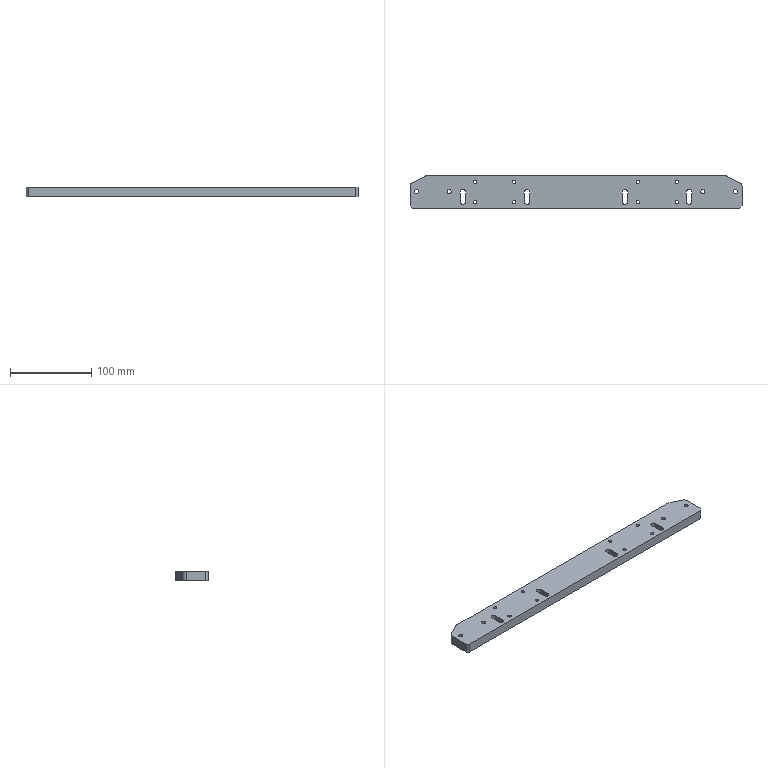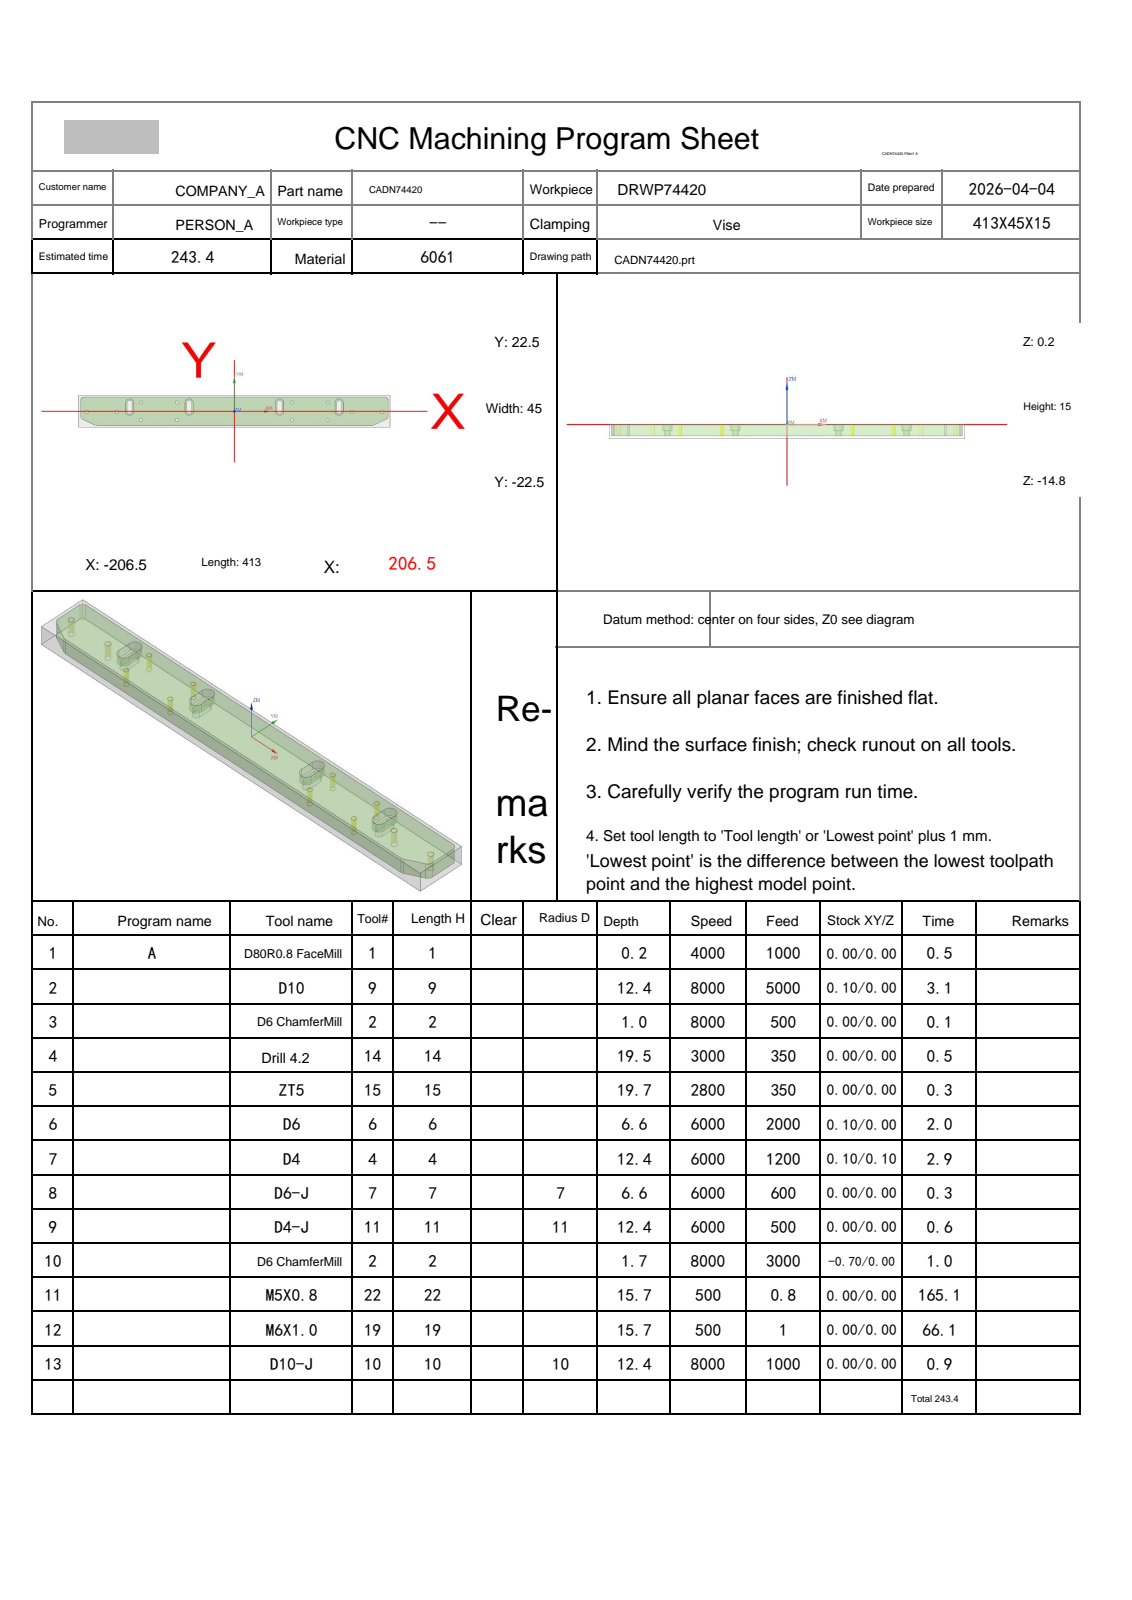NC program | NX | posted by the shop | part box 408 x 40 x 12 mm
Lines 1 to 1071 of 2398:
%
O0001
(Machine time: 462.93 MIN)
(===Total Tool:12===)
(T1=D80R0.8 FaceMill D=80.  R=0.8  D-  H01 Z=0.    )
(T9=D10     D=10.  R=0.   D-  H09 Z=-12.2 )
(T2=D6 ChamferMill   D=6.   R=0.   D-  H02 Z=-1.5  )
(T14=Drill 4.2  D=4.2  DR_a=118 D-  H14 Z=-19.26)
(T15=ZT5    D=5.   DR_a=118 D-  H15 Z=-19.5 )
(T6=D6      D=6.   R=0.   D-  H06 Z=-6.4  )
(T4=D4      D=4.   R=0.   D-  H04 Z=-12.2 )
(T7=D6-J    D=6.   R=0.   D7  H07 Z=-6.4  )
(T11=D4-J   D=4.   R=0.   D11 H11 Z=-12.2 )
(T22=M5X0.8 D=4.2  DR_a=180 D-  H22 Z=-15.5 )
(T19=M6X1.0 D=5.   DR_a=180 D-  H19 Z=-15.5 )
(T10=D10-J  D=10.  R=0.   D10 H10 Z=-12.2 )
G80 G90 G17 G49 G40
G91 G28 Z0
M01
N1 T01 M06
(D80R0.8 FaceMill  D=80. R=0.8 H=01 ce=0.00 di=0.00)
G00 G90 G54 X249. Y0.0 M03 S4000
G43 H01 Z20.
M08
Z2.
G01 Z0.0 F1000.
X244.
X-244.
X-249.
Z2.
G00 Z20.
G91 G28 Z0.0
M05
M09
G91 G28 Z0.0
M01
N2 T09 M06
(D10  D=10. R=0. H=09 ce=0.10 di=0.00)
G00 G90 G54 X0.0 Y25.1 M03 S8000
G43 H09 Z20.
M08
Z.5
G01 X201. Z.324 F5000.
G02 X204.606 Y23.606 Z.321 I0.0 J-5.1
G01 X207.606 Y20.606 Z.317
G02 X209.1 Y17. Z.314 I-3.606 J-3.606
G01 Y-6.91 Z.293
G02 X203.517 Y-15.944 Z.283 I-10.1 J0.0
G01 X187.337 Y-24.034 Z.267
G02 X182.82 Y-25.1 Z.263 I-4.517 J9.034
G01 X-182.82 Z-.057
G02 X-187.337 Y-24.034 Z-.061 I0.0 J10.1
G01 X-203.517 Y-15.944 Z-.077
G02 X-209.1 Y-6.91 Z-.086 I4.517 J9.034
G01 Y17. Z-.107
G02 X-207.606 Y20.606 Z-.111 I5.1 J0.0
G01 X-204.606 Y23.606 Z-.115
G02 X-201. Y25.1 Z-.118 I3.606 J-3.606
G01 X201. Z-.469
G02 X204.606 Y23.606 Z-.473 I0.0 J-5.1
G01 X207.606 Y20.606 Z-.477
G02 X209.1 Y17. Z-.48 I-3.606 J-3.606
G01 Y-6.91 Z-.501
G02 X203.517 Y-15.944 Z-.511 I-10.1 J0.0
G01 X187.337 Y-24.034 Z-.527
G02 X182.82 Y-25.1 Z-.531 I-4.517 J9.034
G01 X-182.82 Z-.85
G02 X-187.337 Y-24.034 Z-.855 I0.0 J10.1
G01 X-203.517 Y-15.944 Z-.87
G02 X-209.1 Y-6.91 Z-.88 I4.517 J9.034
G01 Y17. Z-.901
G02 X-207.606 Y20.606 Z-.905 I5.1 J0.0
G01 X-204.606 Y23.606 Z-.908
G02 X-201. Y25.1 Z-.912 I3.606 J-3.606
G01 X201. Z-1.263
G02 X204.606 Y23.606 Z-1.267 I0.0 J-5.1
G01 X207.606 Y20.606 Z-1.27
G02 X209.1 Y17. Z-1.274 I-3.606 J-3.606
G01 Y-6.91 Z-1.295
G02 X203.517 Y-15.944 Z-1.305 I-10.1 J0.0
G01 X187.337 Y-24.034 Z-1.32
G02 X182.82 Y-25.1 Z-1.325 I-4.517 J9.034
G01 X-182.82 Z-1.644
G02 X-187.337 Y-24.034 Z-1.648 I0.0 J10.1
G01 X-203.517 Y-15.944 Z-1.664
G02 X-209.1 Y-6.91 Z-1.674 I4.517 J9.034
G01 Y17. Z-1.695
G02 X-207.606 Y20.606 Z-1.698 I5.1 J0.0
G01 X-204.606 Y23.606 Z-1.702
G02 X-201. Y25.1 Z-1.706 I3.606 J-3.606
G01 X201. Z-2.057
G02 X204.606 Y23.606 Z-2.06 I0.0 J-5.1
G01 X207.606 Y20.606 Z-2.064
G02 X209.1 Y17. Z-2.068 I-3.606 J-3.606
G01 Y-6.91 Z-2.089
G02 X203.517 Y-15.944 Z-2.098 I-10.1 J0.0
G01 X187.337 Y-24.034 Z-2.114
G02 X182.82 Y-25.1 Z-2.118 I-4.517 J9.034
G01 X-182.82 Z-2.438
G02 X-187.337 Y-24.034 Z-2.442 I0.0 J10.1
G01 X-203.517 Y-15.944 Z-2.458
G02 X-209.1 Y-6.91 Z-2.468 I4.517 J9.034
G01 Y17. Z-2.489
G02 X-207.606 Y20.606 Z-2.492 I5.1 J0.0
G01 X-204.606 Y23.606 Z-2.496
G02 X-201. Y25.1 Z-2.499 I3.606 J-3.606
G01 X201. Z-2.851
G02 X204.606 Y23.606 Z-2.854 I0.0 J-5.1
G01 X207.606 Y20.606 Z-2.858
G02 X209.1 Y17. Z-2.861 I-3.606 J-3.606
G01 Y-6.91 Z-2.882
G02 X203.517 Y-15.944 Z-2.892 I-10.1 J0.0
G01 X187.337 Y-24.034 Z-2.908
G02 X182.82 Y-25.1 Z-2.912 I-4.517 J9.034
G01 X-182.82 Z-3.232
G02 X-187.337 Y-24.034 Z-3.236 I0.0 J10.1
G01 X-203.517 Y-15.944 Z-3.252
G02 X-209.1 Y-6.91 Z-3.261 I4.517 J9.034
G01 Y17. Z-3.282
G02 X-207.606 Y20.606 Z-3.286 I5.1 J0.0
G01 X-204.606 Y23.606 Z-3.29
G02 X-201. Y25.1 Z-3.293 I3.606 J-3.606
G01 X201. Z-3.644
G02 X204.606 Y23.606 Z-3.648 I0.0 J-5.1
G01 X207.606 Y20.606 Z-3.652
G02 X209.1 Y17. Z-3.655 I-3.606 J-3.606
G01 Y-6.91 Z-3.676
G02 X203.517 Y-15.944 Z-3.686 I-10.1 J0.0
G01 X187.337 Y-24.034 Z-3.702
G02 X182.82 Y-25.1 Z-3.706 I-4.517 J9.034
G01 X-182.82 Z-4.025
G02 X-187.337 Y-24.034 Z-4.03 I0.0 J10.1
G01 X-203.517 Y-15.944 Z-4.045
G02 X-209.1 Y-6.91 Z-4.055 I4.517 J9.034
G01 Y17. Z-4.076
G02 X-207.606 Y20.606 Z-4.08 I5.1 J0.0
G01 X-204.606 Y23.606 Z-4.083
G02 X-201. Y25.1 Z-4.087 I3.606 J-3.606
G01 X201. Z-4.438
G02 X204.606 Y23.606 Z-4.442 I0.0 J-5.1
G01 X207.606 Y20.606 Z-4.445
G02 X209.1 Y17. Z-4.449 I-3.606 J-3.606
G01 Y-6.91 Z-4.47
G02 X203.517 Y-15.944 Z-4.48 I-10.1 J0.0
G01 X187.337 Y-24.034 Z-4.495
G02 X182.82 Y-25.1 Z-4.5 I-4.517 J9.034
G01 X-182.82 Z-4.819
G02 X-187.337 Y-24.034 Z-4.823 I0.0 J10.1
G01 X-203.517 Y-15.944 Z-4.839
G02 X-209.1 Y-6.91 Z-4.849 I4.517 J9.034
G01 Y17. Z-4.87
G02 X-207.606 Y20.606 Z-4.873 I5.1 J0.0
G01 X-204.606 Y23.606 Z-4.877
G02 X-201. Y25.1 Z-4.881 I3.606 J-3.606
G01 X201. Z-5.232
G02 X204.606 Y23.606 Z-5.235 I0.0 J-5.1
G01 X207.606 Y20.606 Z-5.239
G02 X209.1 Y17. Z-5.243 I-3.606 J-3.606
G01 Y-6.91 Z-5.264
G02 X203.517 Y-15.944 Z-5.273 I-10.1 J0.0
G01 X187.337 Y-24.034 Z-5.289
G02 X182.82 Y-25.1 Z-5.293 I-4.517 J9.034
G01 X-182.82 Z-5.613
G02 X-187.337 Y-24.034 Z-5.617 I0.0 J10.1
G01 X-203.517 Y-15.944 Z-5.633
G02 X-209.1 Y-6.91 Z-5.643 I4.517 J9.034
G01 Y17. Z-5.664
G02 X-207.606 Y20.606 Z-5.667 I5.1 J0.0
G01 X-204.606 Y23.606 Z-5.671
G02 X-201. Y25.1 Z-5.674 I3.606 J-3.606
G01 X201. Z-6.026
G02 X204.606 Y23.606 Z-6.029 I0.0 J-5.1
G01 X207.606 Y20.606 Z-6.033
G02 X209.1 Y17. Z-6.036 I-3.606 J-3.606
G01 Y-6.91 Z-6.057
G02 X203.517 Y-15.944 Z-6.067 I-10.1 J0.0
G01 X187.337 Y-24.034 Z-6.083
G02 X182.82 Y-25.1 Z-6.087 I-4.517 J9.034
G01 X-182.82 Z-6.407
G02 X-187.337 Y-24.034 Z-6.411 I0.0 J10.1
G01 X-203.517 Y-15.944 Z-6.427
G02 X-209.1 Y-6.91 Z-6.436 I4.517 J9.034
G01 Y17. Z-6.457
G02 X-207.606 Y20.606 Z-6.461 I5.1 J0.0
G01 X-204.606 Y23.606 Z-6.465
G02 X-201. Y25.1 Z-6.468 I3.606 J-3.606
G01 X201. Z-6.819
G02 X204.606 Y23.606 Z-6.823 I0.0 J-5.1
G01 X207.606 Y20.606 Z-6.827
G02 X209.1 Y17. Z-6.83 I-3.606 J-3.606
G01 Y-6.91 Z-6.851
G02 X203.517 Y-15.944 Z-6.861 I-10.1 J0.0
G01 X187.337 Y-24.034 Z-6.877
G02 X182.82 Y-25.1 Z-6.881 I-4.517 J9.034
G01 X-182.82 Z-7.2
G02 X-187.337 Y-24.034 Z-7.205 I0.0 J10.1
G01 X-203.517 Y-15.944 Z-7.22
G02 X-209.1 Y-6.91 Z-7.23 I4.517 J9.034
G01 Y17. Z-7.251
G02 X-207.606 Y20.606 Z-7.255 I5.1 J0.0
G01 X-204.606 Y23.606 Z-7.258
G02 X-201. Y25.1 Z-7.262 I3.606 J-3.606
G01 X201. Z-7.613
G02 X204.606 Y23.606 Z-7.617 I0.0 J-5.1
G01 X207.606 Y20.606 Z-7.62
G02 X209.1 Y17. Z-7.624 I-3.606 J-3.606
G01 Y-6.91 Z-7.645
G02 X203.517 Y-15.944 Z-7.655 I-10.1 J0.0
G01 X187.337 Y-24.034 Z-7.67
G02 X182.82 Y-25.1 Z-7.675 I-4.517 J9.034
G01 X-182.82 Z-7.994
G02 X-187.337 Y-24.034 Z-7.998 I0.0 J10.1
G01 X-203.517 Y-15.944 Z-8.014
G02 X-209.1 Y-6.91 Z-8.024 I4.517 J9.034
G01 Y17. Z-8.045
G02 X-207.606 Y20.606 Z-8.048 I5.1 J0.0
G01 X-204.606 Y23.606 Z-8.052
G02 X-201. Y25.1 Z-8.056 I3.606 J-3.606
G01 X201. Z-8.407
G02 X204.606 Y23.606 Z-8.41 I0.0 J-5.1
G01 X207.606 Y20.606 Z-8.414
G02 X209.1 Y17. Z-8.418 I-3.606 J-3.606
G01 Y-6.91 Z-8.439
G02 X203.517 Y-15.944 Z-8.448 I-10.1 J0.0
G01 X187.337 Y-24.034 Z-8.464
G02 X182.82 Y-25.1 Z-8.468 I-4.517 J9.034
G01 X-182.82 Z-8.788
G02 X-187.337 Y-24.034 Z-8.792 I0.0 J10.1
G01 X-203.517 Y-15.944 Z-8.808
G02 X-209.1 Y-6.91 Z-8.818 I4.517 J9.034
G01 Y17. Z-8.839
G02 X-207.606 Y20.606 Z-8.842 I5.1 J0.0
G01 X-204.606 Y23.606 Z-8.846
G02 X-201. Y25.1 Z-8.849 I3.606 J-3.606
G01 X201. Z-9.201
G02 X204.606 Y23.606 Z-9.204 I0.0 J-5.1
G01 X207.606 Y20.606 Z-9.208
G02 X209.1 Y17. Z-9.211 I-3.606 J-3.606
G01 Y-6.91 Z-9.232
G02 X203.517 Y-15.944 Z-9.242 I-10.1 J0.0
G01 X187.337 Y-24.034 Z-9.258
G02 X182.82 Y-25.1 Z-9.262 I-4.517 J9.034
G01 X-182.82 Z-9.582
G02 X-187.337 Y-24.034 Z-9.586 I0.0 J10.1
G01 X-203.517 Y-15.944 Z-9.602
G02 X-209.1 Y-6.91 Z-9.611 I4.517 J9.034
G01 Y17. Z-9.632
G02 X-207.606 Y20.606 Z-9.636 I5.1 J0.0
G01 X-204.606 Y23.606 Z-9.64
G02 X-201. Y25.1 Z-9.643 I3.606 J-3.606
G01 X201. Z-9.994
G02 X204.606 Y23.606 Z-9.998 I0.0 J-5.1
G01 X207.606 Y20.606 Z-10.002
G02 X209.1 Y17. Z-10.005 I-3.606 J-3.606
G01 Y-6.91 Z-10.026
G02 X203.517 Y-15.944 Z-10.036 I-10.1 J0.0
G01 X187.337 Y-24.034 Z-10.052
G02 X182.82 Y-25.1 Z-10.056 I-4.517 J9.034
G01 X-182.82 Z-10.375
G02 X-187.337 Y-24.034 Z-10.38 I0.0 J10.1
G01 X-203.517 Y-15.944 Z-10.395
G02 X-209.1 Y-6.91 Z-10.405 I4.517 J9.034
G01 Y17. Z-10.426
G02 X-207.606 Y20.606 Z-10.43 I5.1 J0.0
G01 X-204.606 Y23.606 Z-10.433
G02 X-201. Y25.1 Z-10.437 I3.606 J-3.606
G01 X201. Z-10.788
G02 X204.606 Y23.606 Z-10.792 I0.0 J-5.1
G01 X207.606 Y20.606 Z-10.795
G02 X209.1 Y17. Z-10.799 I-3.606 J-3.606
G01 Y-6.91 Z-10.82
G02 X203.517 Y-15.944 Z-10.83 I-10.1 J0.0
G01 X187.337 Y-24.034 Z-10.845
G02 X182.82 Y-25.1 Z-10.85 I-4.517 J9.034
G01 X-182.82 Z-11.169
G02 X-187.337 Y-24.034 Z-11.173 I0.0 J10.1
G01 X-203.517 Y-15.944 Z-11.189
G02 X-209.1 Y-6.91 Z-11.199 I4.517 J9.034
G01 Y17. Z-11.22
G02 X-207.606 Y20.606 Z-11.223 I5.1 J0.0
G01 X-204.606 Y23.606 Z-11.227
G02 X-201. Y25.1 Z-11.231 I3.606 J-3.606
G01 X201. Z-11.582
G02 X204.606 Y23.606 Z-11.585 I0.0 J-5.1
G01 X207.606 Y20.606 Z-11.589
G02 X209.1 Y17. Z-11.593 I-3.606 J-3.606
G01 Y-6.91 Z-11.614
G02 X203.517 Y-15.944 Z-11.623 I-10.1 J0.0
G01 X187.337 Y-24.034 Z-11.639
G02 X182.82 Y-25.1 Z-11.643 I-4.517 J9.034
G01 X-182.82 Z-11.963
G02 X-187.337 Y-24.034 Z-11.967 I0.0 J10.1
G01 X-203.517 Y-15.944 Z-11.983
G02 X-209.1 Y-6.91 Z-11.993 I4.517 J9.034
G01 Y17. Z-12.014
G02 X-207.606 Y20.606 Z-12.017 I5.1 J0.0
G01 X-204.606 Y23.606 Z-12.021
G02 X-201. Y25.1 Z-12.024 I3.606 J-3.606
G01 X0.0 Z-12.2
X201.
G02 X204.606 Y23.606 I0.0 J-5.1
G01 X207.606 Y20.606
G02 X209.1 Y17. I-3.606 J-3.606
G01 Y-6.91
G02 X203.517 Y-15.944 I-10.1 J0.0
G01 X187.337 Y-24.034
G02 X182.82 Y-25.1 I-4.517 J9.034
G01 X-182.82
G02 X-187.337 Y-24.034 I0.0 J10.1
G01 X-203.517 Y-15.944
G02 X-209.1 Y-6.91 I4.517 J9.034
G01 Y17.
G02 X-207.606 Y20.606 I5.1 J0.0
G01 X-204.606 Y23.606
G02 X-201. Y25.1 I3.606 J-3.606
G01 X0.0
X.5
Z-11.2
G00 Z20.
G91 G28 Z0.0
M05
M09
G91 G28 Z0.0
M01
N3 T02 M06
(D6 ChamferMill  D=6. R=0. H=02 ce=0.00 di=0.00)
G00 G90 G54 X-196. Y-.5 M03 S8000
G43 H02 Z20.
M08
G98 G81 X-196. Y-.5 Z-.8 R1. F500.
X-156.
X-124. Y12.5
Y-12.5
X-76.
Y12.5
X76.
Y-12.5
X124.
Y12.5
X156. Y-.5
X196.
G80
G00 Z20.
G91 G28 Z0.0
M05
M09
G91 G28 Z0.0
M01
N4 T14 M06
(Drill 4.2 D=4.2 DR_a=118 H=14)
G00 G90 G54 X124. Y-12.5 M03 S3000
G43 H14 Z20.
M08
G98 G83 X124. Y-12.5 Z-19.262 R1. F350. Q3.
Y12.5
X76.
Y-12.5
X-76.
Y12.5
X-124.
Y-12.5
G80
G00 Z20.
G91 G28 Z0.0
M05
M09
G91 G28 Z0.0
M01
N5 T15 M06
(ZT5 D=5. DR_a=118 H=15)
G00 G90 G54 X-196. Y-.5 M03 S2800
G43 H15 Z20.
M08
G98 G83 X-196. Y-.5 Z-19.502 R1. F350. Q3.
X-156.
X156.
X196.
G80
G00 Z20.
G91 G28 Z0.0
M05
M09
G91 G28 Z0.0
M01
N6 T06 M06
(D6  D=6. R=0. H=06 ce=0.10 di=0.00)
G00 G90 G54 X-136.6 Y6. M03 S6000
G43 H06 Z20.
M08
Z.5
G01 Y12. Z.456 F2000.
G03 X-139. Y14.4 Z.428 I-2.4 J0.0
X-140.275 Y14.033 Z.418 I0.0 J-2.4
X-141.4 Y12. Z.4 I1.275 J-2.033
G01 Y0.0 Z.312
G03 X-139. Y-2.4 Z.284 I2.4 J0.0
X-136.6 Y0.0 Z.257 I0.0 J2.4
G01 Y12. Z.168
G03 X-139. Y14.4 Z.141 I-2.4 J0.0
X-140.275 Y14.033 Z.131 I0.0 J-2.4
X-141.4 Y12. Z.113 I1.275 J-2.033
G01 Y0.0 Z.025
G03 X-139. Y-2.4 Z-.003 I2.4 J0.0
X-136.6 Y0.0 Z-.031 I0.0 J2.4
G01 Y12. Z-.119
G03 X-139. Y14.4 Z-.147 I-2.4 J0.0
X-140.275 Y14.033 Z-.157 I0.0 J-2.4
X-141.4 Y12. Z-.175 I1.275 J-2.033
G01 Y0.0 Z-.263
G03 X-139. Y-2.4 Z-.291 I2.4 J0.0
X-136.6 Y0.0 Z-.318 I0.0 J2.4
G01 Y12. Z-.407
G03 X-139. Y14.4 Z-.434 I-2.4 J0.0
X-140.275 Y14.033 Z-.444 I0.0 J-2.4
X-141.4 Y12. Z-.462 I1.275 J-2.033
G01 Y0.0 Z-.55
G03 X-139. Y-2.4 Z-.578 I2.4 J0.0
X-136.6 Y0.0 Z-.606 I0.0 J2.4
G01 Y12. Z-.694
G03 X-139. Y14.4 Z-.722 I-2.4 J0.0
X-140.275 Y14.033 Z-.732 I0.0 J-2.4
X-141.4 Y12. Z-.75 I1.275 J-2.033
G01 Y0.0 Z-.838
G03 X-139. Y-2.4 Z-.866 I2.4 J0.0
X-136.6 Y0.0 Z-.893 I0.0 J2.4
G01 Y12. Z-.982
G03 X-139. Y14.4 Z-1.009 I-2.4 J0.0
X-140.275 Y14.033 Z-1.019 I0.0 J-2.4
X-141.4 Y12. Z-1.037 I1.275 J-2.033
G01 Y0.0 Z-1.125
G03 X-139. Y-2.4 Z-1.153 I2.4 J0.0
X-136.6 Y0.0 Z-1.181 I0.0 J2.4
G01 Y12. Z-1.269
G03 X-139. Y14.4 Z-1.297 I-2.4 J0.0
X-140.275 Y14.033 Z-1.307 I0.0 J-2.4
X-141.4 Y12. Z-1.325 I1.275 J-2.033
G01 Y0.0 Z-1.413
G03 X-139. Y-2.4 Z-1.441 I2.4 J0.0
X-136.6 Y0.0 Z-1.468 I0.0 J2.4
G01 Y12. Z-1.557
G03 X-139. Y14.4 Z-1.584 I-2.4 J0.0
X-140.275 Y14.033 Z-1.594 I0.0 J-2.4
X-141.4 Y12. Z-1.612 I1.275 J-2.033
G01 Y0.0 Z-1.7
G03 X-139. Y-2.4 Z-1.728 I2.4 J0.0
X-136.6 Y0.0 Z-1.756 I0.0 J2.4
G01 Y12. Z-1.844
G03 X-139. Y14.4 Z-1.872 I-2.4 J0.0
X-140.275 Y14.033 Z-1.882 I0.0 J-2.4
X-141.4 Y12. Z-1.9 I1.275 J-2.033
G01 Y0.0 Z-1.988
G03 X-139. Y-2.4 Z-2.016 I2.4 J0.0
X-136.6 Y0.0 Z-2.043 I0.0 J2.4
G01 Y12. Z-2.132
G03 X-139. Y14.4 Z-2.159 I-2.4 J0.0
X-140.275 Y14.033 Z-2.169 I0.0 J-2.4
X-141.4 Y12. Z-2.187 I1.275 J-2.033
G01 Y0.0 Z-2.275
G03 X-139. Y-2.4 Z-2.303 I2.4 J0.0
X-136.6 Y0.0 Z-2.331 I0.0 J2.4
G01 Y12. Z-2.419
G03 X-139. Y14.4 Z-2.447 I-2.4 J0.0
X-140.275 Y14.033 Z-2.457 I0.0 J-2.4
X-141.4 Y12. Z-2.475 I1.275 J-2.033
G01 Y0.0 Z-2.563
G03 X-139. Y-2.4 Z-2.591 I2.4 J0.0
X-136.6 Y0.0 Z-2.618 I0.0 J2.4
G01 Y12. Z-2.707
G03 X-139. Y14.4 Z-2.734 I-2.4 J0.0
X-140.275 Y14.033 Z-2.744 I0.0 J-2.4
X-141.4 Y12. Z-2.762 I1.275 J-2.033
G01 Y0.0 Z-2.85
G03 X-139. Y-2.4 Z-2.878 I2.4 J0.0
X-136.6 Y0.0 Z-2.906 I0.0 J2.4
G01 Y12. Z-2.994
G03 X-139. Y14.4 Z-3.022 I-2.4 J0.0
X-140.275 Y14.033 Z-3.032 I0.0 J-2.4
X-141.4 Y12. Z-3.05 I1.275 J-2.033
G01 Y0.0 Z-3.138
G03 X-139. Y-2.4 Z-3.166 I2.4 J0.0
X-136.6 Y0.0 Z-3.193 I0.0 J2.4
G01 Y12. Z-3.282
G03 X-139. Y14.4 Z-3.309 I-2.4 J0.0
X-140.275 Y14.033 Z-3.319 I0.0 J-2.4
X-141.4 Y12. Z-3.337 I1.275 J-2.033
G01 Y0.0 Z-3.425
G03 X-139. Y-2.4 Z-3.453 I2.4 J0.0
X-136.6 Y0.0 Z-3.481 I0.0 J2.4
G01 Y12. Z-3.569
G03 X-139. Y14.4 Z-3.597 I-2.4 J0.0
X-140.275 Y14.033 Z-3.607 I0.0 J-2.4
X-141.4 Y12. Z-3.625 I1.275 J-2.033
G01 Y0.0 Z-3.713
G03 X-139. Y-2.4 Z-3.741 I2.4 J0.0
X-136.6 Y0.0 Z-3.768 I0.0 J2.4
G01 Y12. Z-3.857
G03 X-139. Y14.4 Z-3.884 I-2.4 J0.0
X-140.275 Y14.033 Z-3.894 I0.0 J-2.4
X-141.4 Y12. Z-3.912 I1.275 J-2.033
G01 Y0.0 Z-4.
G03 X-139. Y-2.4 Z-4.028 I2.4 J0.0
X-136.6 Y0.0 Z-4.056 I0.0 J2.4
G01 Y12. Z-4.144
G03 X-139. Y14.4 Z-4.172 I-2.4 J0.0
X-140.275 Y14.033 Z-4.182 I0.0 J-2.4
X-141.4 Y12. Z-4.2 I1.275 J-2.033
G01 Y0.0 Z-4.288
G03 X-139. Y-2.4 Z-4.316 I2.4 J0.0
X-136.6 Y0.0 Z-4.343 I0.0 J2.4
G01 Y12. Z-4.432
G03 X-139. Y14.4 Z-4.459 I-2.4 J0.0
X-140.275 Y14.033 Z-4.469 I0.0 J-2.4
X-141.4 Y12. Z-4.487 I1.275 J-2.033
G01 Y0.0 Z-4.575
G03 X-139. Y-2.4 Z-4.603 I2.4 J0.0
X-136.6 Y0.0 Z-4.631 I0.0 J2.4
G01 Y12. Z-4.719
G03 X-139. Y14.4 Z-4.747 I-2.4 J0.0
X-140.275 Y14.033 Z-4.757 I0.0 J-2.4
X-141.4 Y12. Z-4.775 I1.275 J-2.033
G01 Y0.0 Z-4.863
G03 X-139. Y-2.4 Z-4.891 I2.4 J0.0
X-136.6 Y0.0 Z-4.918 I0.0 J2.4
G01 Y12. Z-5.007
G03 X-139. Y14.4 Z-5.034 I-2.4 J0.0
X-140.275 Y14.033 Z-5.044 I0.0 J-2.4
X-141.4 Y12. Z-5.062 I1.275 J-2.033
G01 Y0.0 Z-5.15
G03 X-139. Y-2.4 Z-5.178 I2.4 J0.0
X-136.6 Y0.0 Z-5.206 I0.0 J2.4
G01 Y12. Z-5.294
G03 X-139. Y14.4 Z-5.322 I-2.4 J0.0
X-140.275 Y14.033 Z-5.332 I0.0 J-2.4
X-141.4 Y12. Z-5.35 I1.275 J-2.033
G01 Y0.0 Z-5.438
G03 X-139. Y-2.4 Z-5.466 I2.4 J0.0
X-136.6 Y0.0 Z-5.493 I0.0 J2.4
G01 Y12. Z-5.582
G03 X-139. Y14.4 Z-5.609 I-2.4 J0.0
X-140.275 Y14.033 Z-5.619 I0.0 J-2.4
X-141.4 Y12. Z-5.637 I1.275 J-2.033
G01 Y0.0 Z-5.725
G03 X-139. Y-2.4 Z-5.753 I2.4 J0.0
X-136.6 Y0.0 Z-5.781 I0.0 J2.4
G01 Y12. Z-5.869
G03 X-139. Y14.4 Z-5.897 I-2.4 J0.0
X-140.275 Y14.033 Z-5.907 I0.0 J-2.4
X-141.4 Y12. Z-5.925 I1.275 J-2.033
G01 Y0.0 Z-6.013
G03 X-139. Y-2.4 Z-6.041 I2.4 J0.0
X-136.6 Y0.0 Z-6.068 I0.0 J2.4
G01 Y12. Z-6.157
G03 X-139. Y14.4 Z-6.184 I-2.4 J0.0
X-140.275 Y14.033 Z-6.194 I0.0 J-2.4
X-141.4 Y12. Z-6.212 I1.275 J-2.033
G01 Y0.0 Z-6.3
G03 X-139. Y-2.4 Z-6.328 I2.4 J0.0
X-136.6 Y0.0 Z-6.356 I0.0 J2.4
G01 Y6. Z-6.4
Y12.
G03 X-139. Y14.4 I-2.4 J0.0
X-141.4 Y12. I0.0 J-2.4
G01 Y0.0
G03 X-139. Y-2.4 I2.4 J0.0
X-136.6 Y0.0 I0.0 J2.4
G01 Y6.
Y6.5
Z-5.4
G00 Z20.
X-62.4 Y5.816
Z.5
G01 Y0.0 Z.457
G03 X-62.372 Y-.366 Z.455 I2.4 J0.0
X-60. Y-2.4 Z.429 I2.372 J.366
X-57.6 Y0.0 Z.402 I0.0 J2.4
G01 Y12. Z.313
G03 X-60. Y14.4 Z.286 I-2.4 J0.0
X-62.4 Y12. Z.258 I0.0 J-2.4
G01 Y0.0 Z.17
G03 X-62.372 Y-.366 Z.167 I2.4 J0.0
X-60. Y-2.4 Z.142 I2.372 J.366
X-57.6 Y0.0 Z.114 I0.0 J2.4
G01 Y12. Z.026
G03 X-60. Y14.4 Z-.002 I-2.4 J0.0
X-62.4 Y12. Z-.03 I0.0 J-2.4
G01 Y0.0 Z-.118
G03 X-62.372 Y-.366 Z-.12 I2.4 J0.0
X-60. Y-2.4 Z-.146 I2.372 J.366
X-57.6 Y0.0 Z-.173 I0.0 J2.4
G01 Y12. Z-.262
G03 X-60. Y14.4 Z-.289 I-2.4 J0.0
X-62.4 Y12. Z-.317 I0.0 J-2.4
G01 Y0.0 Z-.405
G03 X-62.372 Y-.366 Z-.408 I2.4 J0.0
X-60. Y-2.4 Z-.433 I2.372 J.366
X-57.6 Y0.0 Z-.461 I0.0 J2.4
G01 Y12. Z-.549
G03 X-60. Y14.4 Z-.577 I-2.4 J0.0
X-62.4 Y12. Z-.605 I0.0 J-2.4
G01 Y0.0 Z-.693
G03 X-62.372 Y-.366 Z-.695 I2.4 J0.0
X-60. Y-2.4 Z-.721 I2.372 J.366
X-57.6 Y0.0 Z-.748 I0.0 J2.4
G01 Y12. Z-.837
G03 X-60. Y14.4 Z-.864 I-2.4 J0.0
X-62.4 Y12. Z-.892 I0.0 J-2.4
G01 Y0.0 Z-.98
G03 X-62.372 Y-.366 Z-.983 I2.4 J0.0
X-60. Y-2.4 Z-1.008 I2.372 J.366
X-57.6 Y0.0 Z-1.036 I0.0 J2.4
G01 Y12. Z-1.124
G03 X-60. Y14.4 Z-1.152 I-2.4 J0.0
X-62.4 Y12. Z-1.18 I0.0 J-2.4
G01 Y0.0 Z-1.268
G03 X-62.372 Y-.366 Z-1.27 I2.4 J0.0
X-60. Y-2.4 Z-1.296 I2.372 J.366
X-57.6 Y0.0 Z-1.323 I0.0 J2.4
G01 Y12. Z-1.412
G03 X-60. Y14.4 Z-1.439 I-2.4 J0.0
X-62.4 Y12. Z-1.467 I0.0 J-2.4
G01 Y0.0 Z-1.555
G03 X-62.372 Y-.366 Z-1.558 I2.4 J0.0
X-60. Y-2.4 Z-1.583 I2.372 J.366
X-57.6 Y0.0 Z-1.611 I0.0 J2.4
G01 Y12. Z-1.699
G03 X-60. Y14.4 Z-1.727 I-2.4 J0.0
X-62.4 Y12. Z-1.755 I0.0 J-2.4
G01 Y0.0 Z-1.843
G03 X-62.372 Y-.366 Z-1.845 I2.4 J0.0
X-60. Y-2.4 Z-1.871 I2.372 J.366
X-57.6 Y0.0 Z-1.898 I0.0 J2.4
G01 Y12. Z-1.987
G03 X-60. Y14.4 Z-2.014 I-2.4 J0.0
X-62.4 Y12. Z-2.042 I0.0 J-2.4
G01 Y0.0 Z-2.13
G03 X-62.372 Y-.366 Z-2.133 I2.4 J0.0
X-60. Y-2.4 Z-2.158 I2.372 J.366
X-57.6 Y0.0 Z-2.186 I0.0 J2.4
G01 Y12. Z-2.274
G03 X-60. Y14.4 Z-2.302 I-2.4 J0.0
X-62.4 Y12. Z-2.33 I0.0 J-2.4
G01 Y0.0 Z-2.418
G03 X-62.372 Y-.366 Z-2.42 I2.4 J0.0
X-60. Y-2.4 Z-2.446 I2.372 J.366
X-57.6 Y0.0 Z-2.473 I0.0 J2.4
G01 Y12. Z-2.562
G03 X-60. Y14.4 Z-2.589 I-2.4 J0.0
X-62.4 Y12. Z-2.617 I0.0 J-2.4
G01 Y0.0 Z-2.705
G03 X-62.372 Y-.366 Z-2.708 I2.4 J0.0
X-60. Y-2.4 Z-2.733 I2.372 J.366
X-57.6 Y0.0 Z-2.761 I0.0 J2.4
G01 Y12. Z-2.849
G03 X-60. Y14.4 Z-2.877 I-2.4 J0.0
X-62.4 Y12. Z-2.905 I0.0 J-2.4
G01 Y0.0 Z-2.993
G03 X-62.372 Y-.366 Z-2.995 I2.4 J0.0
X-60. Y-2.4 Z-3.021 I2.372 J.366
X-57.6 Y0.0 Z-3.048 I0.0 J2.4
G01 Y12. Z-3.137
G03 X-60. Y14.4 Z-3.164 I-2.4 J0.0
X-62.4 Y12. Z-3.192 I0.0 J-2.4
G01 Y0.0 Z-3.28
G03 X-62.372 Y-.366 Z-3.283 I2.4 J0.0
X-60. Y-2.4 Z-3.308 I2.372 J.366
X-57.6 Y0.0 Z-3.336 I0.0 J2.4
G01 Y12. Z-3.424
G03 X-60. Y14.4 Z-3.452 I-2.4 J0.0
X-62.4 Y12. Z-3.48 I0.0 J-2.4
G01 Y0.0 Z-3.568
G03 X-62.372 Y-.366 Z-3.57 I2.4 J0.0
X-60. Y-2.4 Z-3.596 I2.372 J.366
X-57.6 Y0.0 Z-3.623 I0.0 J2.4
G01 Y12. Z-3.712
G03 X-60. Y14.4 Z-3.739 I-2.4 J0.0
X-62.4 Y12. Z-3.767 I0.0 J-2.4
G01 Y0.0 Z-3.855
G03 X-62.372 Y-.366 Z-3.858 I2.4 J0.0
X-60. Y-2.4 Z-3.883 I2.372 J.366
X-57.6 Y0.0 Z-3.911 I0.0 J2.4
G01 Y12. Z-3.999
G03 X-60. Y14.4 Z-4.027 I-2.4 J0.0
X-62.4 Y12. Z-4.055 I0.0 J-2.4
G01 Y0.0 Z-4.143
G03 X-62.372 Y-.366 Z-4.145 I2.4 J0.0
X-60. Y-2.4 Z-4.171 I2.372 J.366
X-57.6 Y0.0 Z-4.198 I0.0 J2.4
G01 Y12. Z-4.287
G03 X-60. Y14.4 Z-4.314 I-2.4 J0.0
X-62.4 Y12. Z-4.342 I0.0 J-2.4
G01 Y0.0 Z-4.43
G03 X-62.372 Y-.366 Z-4.433 I2.4 J0.0
X-60. Y-2.4 Z-4.458 I2.372 J.366
X-57.6 Y0.0 Z-4.486 I0.0 J2.4
G01 Y12. Z-4.574
G03 X-60. Y14.4 Z-4.602 I-2.4 J0.0
X-62.4 Y12. Z-4.63 I0.0 J-2.4
G01 Y0.0 Z-4.718
G03 X-62.372 Y-.366 Z-4.72 I2.4 J0.0
X-60. Y-2.4 Z-4.746 I2.372 J.366
X-57.6 Y0.0 Z-4.773 I0.0 J2.4
G01 Y12. Z-4.862
G03 X-60. Y14.4 Z-4.889 I-2.4 J0.0
X-62.4 Y12. Z-4.917 I0.0 J-2.4
G01 Y0.0 Z-5.005
G03 X-62.372 Y-.366 Z-5.008 I2.4 J0.0
X-60. Y-2.4 Z-5.033 I2.372 J.366
X-57.6 Y0.0 Z-5.061 I0.0 J2.4
G01 Y12. Z-5.149
G03 X-60. Y14.4 Z-5.177 I-2.4 J0.0
X-62.4 Y12. Z-5.205 I0.0 J-2.4
G01 Y0.0 Z-5.293
G03 X-62.372 Y-.366 Z-5.295 I2.4 J0.0
X-60. Y-2.4 Z-5.321 I2.372 J.366
X-57.6 Y0.0 Z-5.348 I0.0 J2.4
G01 Y12. Z-5.437
G03 X-60. Y14.4 Z-5.464 I-2.4 J0.0
X-62.4 Y12. Z-5.492 I0.0 J-2.4
G01 Y0.0 Z-5.58
G03 X-62.372 Y-.366 Z-5.583 I2.4 J0.0
X-60. Y-2.4 Z-5.608 I2.372 J.366
X-57.6 Y0.0 Z-5.636 I0.0 J2.4
G01 Y12. Z-5.724
G03 X-60. Y14.4 Z-5.752 I-2.4 J0.0
X-62.4 Y12. Z-5.78 I0.0 J-2.4
G01 Y0.0 Z-5.868
G03 X-62.372 Y-.366 Z-5.87 I2.4 J0.0
X-60. Y-2.4 Z-5.896 I2.372 J.366
X-57.6 Y0.0 Z-5.923 I0.0 J2.4
G01 Y12. Z-6.012
G03 X-60. Y14.4 Z-6.039 I-2.4 J0.0
X-62.4 Y12. Z-6.067 I0.0 J-2.4
G01 Y0.0 Z-6.155
G03 X-62.372 Y-.366 Z-6.158 I2.4 J0.0
X-60. Y-2.4 Z-6.183 I2.372 J.366
X-57.6 Y0.0 Z-6.211 I0.0 J2.4
G01 Y12. Z-6.299
G03 X-60. Y14.4 Z-6.327 I-2.4 J0.0
X-62.4 Y12. Z-6.355 I0.0 J-2.4
G01 Y5.816 Z-6.4
Y0.0
G03 X-60. Y-2.4 I2.4 J0.0
X-57.6 Y0.0 I0.0 J2.4
G01 Y12.
G03 X-60. Y14.4 I-2.4 J0.0
X-62.4 Y12. I0.0 J-2.4
G01 Y5.816
Y5.316
Z-5.4
G00 Z20.
X57.6 Y6.
Z.5
G01 Y0.0 Z.456
G03 X60. Y-2.4 Z.428 I2.4 J0.0
X62.4 Y0.0 Z.4 I0.0 J2.4
G01 Y12. Z.312
G03 X60. Y14.4 Z.284 I-2.4 J0.0
X57.6 Y12. Z.257 I0.0 J-2.4
G01 Y0.0 Z.168
G03 X60. Y-2.4 Z.141 I2.4 J0.0
X62.4 Y0.0 Z.113 I0.0 J2.4
G01 Y12. Z.025
G03 X60. Y14.4 Z-.003 I-2.4 J0.0
X57.6 Y12. Z-.031 I0.0 J-2.4
G01 Y0.0 Z-.119
G03 X60. Y-2.4 Z-.147 I2.4 J0.0
X62.4 Y0.0 Z-.175 I0.0 J2.4
G01 Y12. Z-.263
G03 X60. Y14.4 Z-.291 I-2.4 J0.0
X57.6 Y12. Z-.318 I0.0 J-2.4
G01 Y0.0 Z-.407
G03 X60. Y-2.4 Z-.434 I2.4 J0.0
X62.4 Y0.0 Z-.462 I0.0 J2.4
G01 Y12. Z-.55
G03 X60. Y14.4 Z-.578 I-2.4 J0.0
X57.6 Y12. Z-.606 I0.0 J-2.4
G01 Y0.0 Z-.694
G03 X60. Y-2.4 Z-.722 I2.4 J0.0
X62.4 Y0.0 Z-.75 I0.0 J2.4
G01 Y12. Z-.838
G03 X60. Y14.4 Z-.866 I-2.4 J0.0
X57.6 Y12. Z-.893 I0.0 J-2.4
G01 Y0.0 Z-.982
G03 X60. Y-2.4 Z-1.009 I2.4 J0.0
X62.4 Y0.0 Z-1.037 I0.0 J2.4
G01 Y12. Z-1.125
G03 X60. Y14.4 Z-1.153 I-2.4 J0.0
X57.6 Y12. Z-1.181 I0.0 J-2.4
G01 Y0.0 Z-1.269
G03 X60. Y-2.4 Z-1.297 I2.4 J0.0
X62.4 Y0.0 Z-1.325 I0.0 J2.4
G01 Y12. Z-1.413
G03 X60. Y14.4 Z-1.441 I-2.4 J0.0
X57.6 Y12. Z-1.468 I0.0 J-2.4
G01 Y0.0 Z-1.557
G03 X60. Y-2.4 Z-1.584 I2.4 J0.0
X62.4 Y0.0 Z-1.612 I0.0 J2.4
G01 Y12. Z-1.7
G03 X60. Y14.4 Z-1.728 I-2.4 J0.0
X57.6 Y12. Z-1.756 I0.0 J-2.4
G01 Y0.0 Z-1.844
G03 X60. Y-2.4 Z-1.872 I2.4 J0.0
X62.4 Y0.0 Z-1.9 I0.0 J2.4
G01 Y12. Z-1.988
G03 X60. Y14.4 Z-2.016 I-2.4 J0.0
X57.6 Y12. Z-2.043 I0.0 J-2.4
G01 Y0.0 Z-2.132
G03 X60. Y-2.4 Z-2.159 I2.4 J0.0
X62.4 Y0.0 Z-2.187 I0.0 J2.4
G01 Y12. Z-2.275
G03 X60. Y14.4 Z-2.303 I-2.4 J0.0
X57.6 Y12. Z-2.331 I0.0 J-2.4
G01 Y0.0 Z-2.419
G03 X60. Y-2.4 Z-2.447 I2.4 J0.0
X62.4 Y0.0 Z-2.475 I0.0 J2.4
G01 Y12. Z-2.563
G03 X60. Y14.4 Z-2.591 I-2.4 J0.0
X57.6 Y12. Z-2.618 I0.0 J-2.4
G01 Y0.0 Z-2.707
G03 X60. Y-2.4 Z-2.734 I2.4 J0.0
X62.4 Y0.0 Z-2.762 I0.0 J2.4
G01 Y12. Z-2.85
G03 X60. Y14.4 Z-2.878 I-2.4 J0.0
X57.6 Y12. Z-2.906 I0.0 J-2.4
G01 Y0.0 Z-2.994
G03 X60. Y-2.4 Z-3.022 I2.4 J0.0
X62.4 Y0.0 Z-3.05 I0.0 J2.4
G01 Y12. Z-3.138
G03 X60. Y14.4 Z-3.166 I-2.4 J0.0
X57.6 Y12. Z-3.193 I0.0 J-2.4
G01 Y0.0 Z-3.282
G03 X60. Y-2.4 Z-3.309 I2.4 J0.0
X62.4 Y0.0 Z-3.337 I0.0 J2.4
G01 Y12. Z-3.425
G03 X60. Y14.4 Z-3.453 I-2.4 J0.0
X57.6 Y12. Z-3.481 I0.0 J-2.4
G01 Y0.0 Z-3.569
G03 X60. Y-2.4 Z-3.597 I2.4 J0.0
X62.4 Y0.0 Z-3.625 I0.0 J2.4
G01 Y12. Z-3.713
G03 X60. Y14.4 Z-3.741 I-2.4 J0.0
X57.6 Y12. Z-3.768 I0.0 J-2.4
G01 Y0.0 Z-3.857
G03 X60. Y-2.4 Z-3.884 I2.4 J0.0
X62.4 Y0.0 Z-3.912 I0.0 J2.4
G01 Y12. Z-4.
G03 X60. Y14.4 Z-4.028 I-2.4 J0.0
X57.6 Y12. Z-4.056 I0.0 J-2.4
G01 Y0.0 Z-4.144
G03 X60. Y-2.4 Z-4.172 I2.4 J0.0
X62.4 Y0.0 Z-4.2 I0.0 J2.4
G01 Y12. Z-4.288
G03 X60. Y14.4 Z-4.316 I-2.4 J0.0
X57.6 Y12. Z-4.343 I0.0 J-2.4
G01 Y0.0 Z-4.432
G03 X60. Y-2.4 Z-4.459 I2.4 J0.0
X62.4 Y0.0 Z-4.487 I0.0 J2.4
G01 Y12. Z-4.575
G03 X60. Y14.4 Z-4.603 I-2.4 J0.0
X57.6 Y12. Z-4.631 I0.0 J-2.4
G01 Y0.0 Z-4.719
G03 X60. Y-2.4 Z-4.747 I2.4 J0.0
X62.4 Y0.0 Z-4.775 I0.0 J2.4
G01 Y12. Z-4.863
G03 X60. Y14.4 Z-4.891 I-2.4 J0.0
X57.6 Y12. Z-4.918 I0.0 J-2.4
G01 Y0.0 Z-5.007
G03 X60. Y-2.4 Z-5.034 I2.4 J0.0
X62.4 Y0.0 Z-5.062 I0.0 J2.4
G01 Y12. Z-5.15
G03 X60. Y14.4 Z-5.178 I-2.4 J0.0
X57.6 Y12. Z-5.206 I0.0 J-2.4
G01 Y0.0 Z-5.294
G03 X60. Y-2.4 Z-5.322 I2.4 J0.0
X62.4 Y0.0 Z-5.35 I0.0 J2.4
G01 Y12. Z-5.438
G03 X60. Y14.4 Z-5.466 I-2.4 J0.0
X57.6 Y12. Z-5.493 I0.0 J-2.4
G01 Y0.0 Z-5.582
G03 X60. Y-2.4 Z-5.609 I2.4 J0.0
X62.4 Y0.0 Z-5.637 I0.0 J2.4
G01 Y12. Z-5.725
G03 X60. Y14.4 Z-5.753 I-2.4 J0.0
X57.6 Y12. Z-5.781 I0.0 J-2.4
G01 Y0.0 Z-5.869
G03 X60. Y-2.4 Z-5.897 I2.4 J0.0
X62.4 Y0.0 Z-5.925 I0.0 J2.4
G01 Y12. Z-6.013
G03 X60. Y14.4 Z-6.041 I-2.4 J0.0
X57.6 Y12. Z-6.068 I0.0 J-2.4
G01 Y0.0 Z-6.157
G03 X60. Y-2.4 Z-6.184 I2.4 J0.0
X62.4 Y0.0 Z-6.212 I0.0 J2.4
G01 Y12. Z-6.3
G03 X60. Y14.4 Z-6.328 I-2.4 J0.0
X57.6 Y12. Z-6.356 I0.0 J-2.4
G01 Y6. Z-6.4
Y0.0
G03 X60. Y-2.4 I2.4 J0.0
X62.4 Y0.0 I0.0 J2.4
G01 Y12.
G03 X60. Y14.4 I-2.4 J0.0
X57.6 Y12. I0.0 J-2.4
G01 Y6.
Y5.5
Z-5.4
G00 Z20.
X136.6 Y6.
Z.5
G01 Y0.0 Z.456
G03 X139. Y-2.4 Z.428 I2.4 J0.0
X141.4 Y0.0 Z.4 I0.0 J2.4
G01 Y12. Z.312
G03 X139. Y14.4 Z.284 I-2.4 J0.0
X136.6 Y12. Z.257 I0.0 J-2.4
G01 Y0.0 Z.168
G03 X139. Y-2.4 Z.141 I2.4 J0.0
X141.4 Y0.0 Z.113 I0.0 J2.4
G01 Y12. Z.025
G03 X139. Y14.4 Z-.003 I-2.4 J0.0
X136.6 Y12. Z-.031 I0.0 J-2.4
G01 Y0.0 Z-.119
G03 X139. Y-2.4 Z-.147 I2.4 J0.0
X141.4 Y0.0 Z-.175 I0.0 J2.4
G01 Y12. Z-.263
G03 X139. Y14.4 Z-.291 I-2.4 J0.0
X136.6 Y12. Z-.318 I0.0 J-2.4
G01 Y0.0 Z-.407
G03 X139. Y-2.4 Z-.434 I2.4 J0.0
X141.4 Y0.0 Z-.462 I0.0 J2.4
G01 Y12. Z-.55
G03 X139. Y14.4 Z-.578 I-2.4 J0.0
X136.6 Y12. Z-.606 I0.0 J-2.4
G01 Y0.0 Z-.694
G03 X139. Y-2.4 Z-.722 I2.4 J0.0
X141.4 Y0.0 Z-.75 I0.0 J2.4
G01 Y12. Z-.838
G03 X139. Y14.4 Z-.866 I-2.4 J0.0
X136.6 Y12. Z-.893 I0.0 J-2.4
G01 Y0.0 Z-.982
G03 X139. Y-2.4 Z-1.009 I2.4 J0.0
X141.4 Y0.0 Z-1.037 I0.0 J2.4
G01 Y12. Z-1.125
G03 X139. Y14.4 Z-1.153 I-2.4 J0.0
X136.6 Y12. Z-1.181 I0.0 J-2.4
G01 Y0.0 Z-1.269
G03 X139. Y-2.4 Z-1.297 I2.4 J0.0
X141.4 Y0.0 Z-1.325 I0.0 J2.4
G01 Y12. Z-1.413
G03 X139. Y14.4 Z-1.441 I-2.4 J0.0
X136.6 Y12. Z-1.468 I0.0 J-2.4
G01 Y0.0 Z-1.557
G03 X139. Y-2.4 Z-1.584 I2.4 J0.0
X141.4 Y0.0 Z-1.612 I0.0 J2.4
G01 Y12. Z-1.7
G03 X139. Y14.4 Z-1.728 I-2.4 J0.0
X136.6 Y12. Z-1.756 I0.0 J-2.4
G01 Y0.0 Z-1.844
G03 X139. Y-2.4 Z-1.872 I2.4 J0.0
X141.4 Y0.0 Z-1.9 I0.0 J2.4
G01 Y12. Z-1.988
G03 X139. Y14.4 Z-2.016 I-2.4 J0.0
X136.6 Y12. Z-2.043 I0.0 J-2.4
G01 Y0.0 Z-2.132
G03 X139. Y-2.4 Z-2.159 I2.4 J0.0
X141.4 Y0.0 Z-2.187 I0.0 J2.4
G01 Y12. Z-2.275
G03 X139. Y14.4 Z-2.303 I-2.4 J0.0
X136.6 Y12. Z-2.331 I0.0 J-2.4
G01 Y0.0 Z-2.419
G03 X139. Y-2.4 Z-2.447 I2.4 J0.0
X141.4 Y0.0 Z-2.475 I0.0 J2.4
G01 Y12. Z-2.563
G03 X139. Y14.4 Z-2.591 I-2.4 J0.0
X136.6 Y12. Z-2.618 I0.0 J-2.4
G01 Y0.0 Z-2.707
G03 X139. Y-2.4 Z-2.734 I2.4 J0.0
X141.4 Y0.0 Z-2.762 I0.0 J2.4
G01 Y12. Z-2.85
G03 X139. Y14.4 Z-2.878 I-2.4 J0.0
X136.6 Y12. Z-2.906 I0.0 J-2.4
G01 Y0.0 Z-2.994
G03 X139. Y-2.4 Z-3.022 I2.4 J0.0
X141.4 Y0.0 Z-3.05 I0.0 J2.4
G01 Y12. Z-3.138
G03 X139. Y14.4 Z-3.166 I-2.4 J0.0
X136.6 Y12. Z-3.193 I0.0 J-2.4
G01 Y0.0 Z-3.282
G03 X139. Y-2.4 Z-3.309 I2.4 J0.0
X141.4 Y0.0 Z-3.337 I0.0 J2.4
G01 Y12. Z-3.425
G03 X139. Y14.4 Z-3.453 I-2.4 J0.0
X136.6 Y12. Z-3.481 I0.0 J-2.4
G01 Y0.0 Z-3.569
G03 X139. Y-2.4 Z-3.597 I2.4 J0.0
X141.4 Y0.0 Z-3.625 I0.0 J2.4
G01 Y12. Z-3.713
G03 X139. Y14.4 Z-3.741 I-2.4 J0.0
X136.6 Y12. Z-3.768 I0.0 J-2.4
G01 Y0.0 Z-3.857
G03 X139. Y-2.4 Z-3.884 I2.4 J0.0
X141.4 Y0.0 Z-3.912 I0.0 J2.4
G01 Y12. Z-4.
G03 X139. Y14.4 Z-4.028 I-2.4 J0.0
X136.6 Y12. Z-4.056 I0.0 J-2.4
G01 Y0.0 Z-4.144
G03 X139. Y-2.4 Z-4.172 I2.4 J0.0
X141.4 Y0.0 Z-4.2 I0.0 J2.4
G01 Y12. Z-4.288
G03 X139. Y14.4 Z-4.316 I-2.4 J0.0
X136.6 Y12. Z-4.343 I0.0 J-2.4
G01 Y0.0 Z-4.432
G03 X139. Y-2.4 Z-4.459 I2.4 J0.0
X141.4 Y0.0 Z-4.487 I0.0 J2.4
G01 Y12. Z-4.575
G03 X139. Y14.4 Z-4.603 I-2.4 J0.0
X136.6 Y12. Z-4.631 I0.0 J-2.4
G01 Y0.0 Z-4.719
G03 X139. Y-2.4 Z-4.747 I2.4 J0.0
X141.4 Y0.0 Z-4.775 I0.0 J2.4
G01 Y12. Z-4.863
G03 X139. Y14.4 Z-4.891 I-2.4 J0.0
X136.6 Y12. Z-4.918 I0.0 J-2.4
G01 Y0.0 Z-5.007
G03 X139. Y-2.4 Z-5.034 I2.4 J0.0
X141.4 Y0.0 Z-5.062 I0.0 J2.4
G01 Y12. Z-5.15
G03 X139. Y14.4 Z-5.178 I-2.4 J0.0
X136.6 Y12. Z-5.206 I0.0 J-2.4
G01 Y0.0 Z-5.294
G03 X139. Y-2.4 Z-5.322 I2.4 J0.0
X141.4 Y0.0 Z-5.35 I0.0 J2.4
G01 Y12. Z-5.438
G03 X139. Y14.4 Z-5.466 I-2.4 J0.0
X136.6 Y12. Z-5.493 I0.0 J-2.4
G01 Y0.0 Z-5.582
G03 X139. Y-2.4 Z-5.609 I2.4 J0.0
X141.4 Y0.0 Z-5.637 I0.0 J2.4
G01 Y12. Z-5.725
G03 X139. Y14.4 Z-5.753 I-2.4 J0.0
X136.6 Y12. Z-5.781 I0.0 J-2.4
G01 Y0.0 Z-5.869
G03 X139. Y-2.4 Z-5.897 I2.4 J0.0
X141.4 Y0.0 Z-5.925 I0.0 J2.4
G01 Y12. Z-6.013
G03 X139. Y14.4 Z-6.041 I-2.4 J0.0
X136.6 Y12. Z-6.068 I0.0 J-2.4
G01 Y0.0 Z-6.157
G03 X139. Y-2.4 Z-6.184 I2.4 J0.0
X141.4 Y0.0 Z-6.212 I0.0 J2.4
G01 Y12. Z-6.3
G03 X139. Y14.4 Z-6.328 I-2.4 J0.0
X136.6 Y12. Z-6.356 I0.0 J-2.4
G01 Y6. Z-6.4
Y0.0
G03 X139. Y-2.4 I2.4 J0.0
X141.4 Y0.0 I0.0 J2.4
G01 Y12.
G03 X139. Y14.4 I-2.4 J0.0
X136.6 Y12. I0.0 J-2.4
G01 Y6.
Y5.5
Z-5.4
G00 Z20.
G91 G28 Z0.0
M05
M09
G91 G28 Z0.0
M01